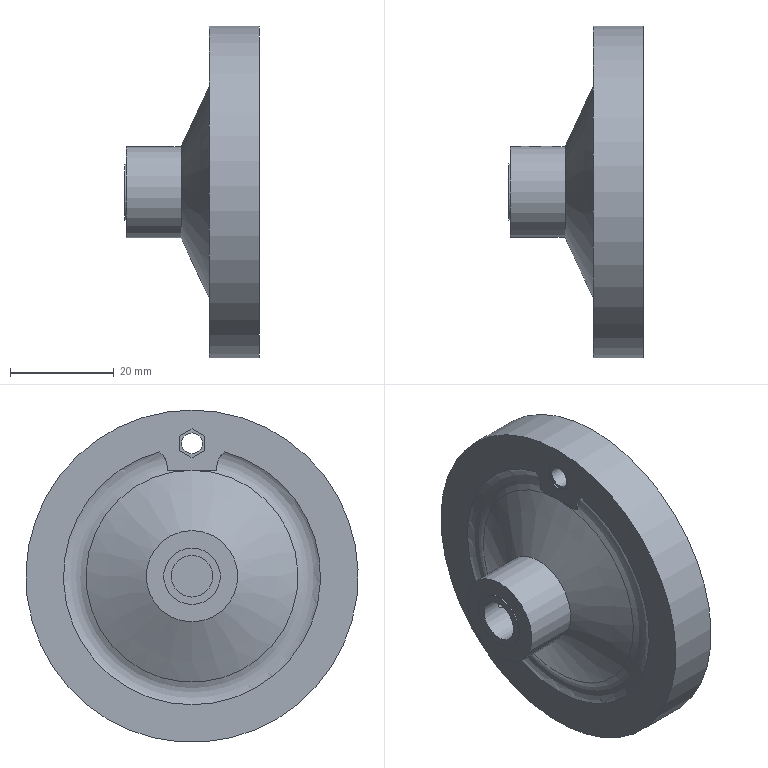Part | NX | features BREP 1 | 1 solid | 38 faces | box 25.84 x 64 x 64 mm | volume 22076 mm3 | plane 22 | cylinder 12 | torus 2 | cone 2 | commonest cylinder face diameters 8 x5 2.4 x1 4 x1 10.88 x1 12.8 x1 17.6 x1
STEP:
#1=CARTESIAN_POINT('',(-9.6,0.,22.829));
#2=VERTEX_POINT('',#1);
#3=CARTESIAN_POINT('',(-9.6,2.4,24.214));
#4=VERTEX_POINT('',#3);
#5=CARTESIAN_POINT('',(-9.6,3.971,25.122));
#6=DIRECTION('',(0.,0.866,0.5));
#7=VECTOR('',#6,1000.);
#8=LINE('',#5,#7);
#9=EDGE_CURVE('',#2,#4,#8,.T.);
#10=ORIENTED_EDGE('',*,*,#9,.F.);
#11=CARTESIAN_POINT('',(-9.36,0.,22.829));
#12=VERTEX_POINT('',#11);
#13=CARTESIAN_POINT('',(-9.36,0.,22.829));
#14=DIRECTION('',(-1.,0.,0.));
#15=VECTOR('',#14,1000.);
#16=LINE('',#13,#15);
#17=EDGE_CURVE('',#12,#2,#16,.T.);
#18=ORIENTED_EDGE('',*,*,#17,.F.);
#19=CARTESIAN_POINT('',(-9.36,2.4,24.214));
#20=VERTEX_POINT('',#19);
#21=CARTESIAN_POINT('',(-9.36,0.,22.829));
#22=DIRECTION('',(0.,0.866,0.5));
#23=VECTOR('',#22,1000.);
#24=LINE('',#21,#23);
#25=EDGE_CURVE('',#12,#20,#24,.T.);
#26=ORIENTED_EDGE('',*,*,#25,.T.);
#27=CARTESIAN_POINT('',(-9.36,2.4,24.214));
#28=DIRECTION('',(-1.,0.,0.));
#29=VECTOR('',#28,1000.);
#30=LINE('',#27,#29);
#31=EDGE_CURVE('',#20,#4,#30,.T.);
#32=ORIENTED_EDGE('',*,*,#31,.T.);
#33=EDGE_LOOP('',(#10,#18,#26,#32));
#34=FACE_BOUND('',#33,.T.);
#35=CARTESIAN_POINT('',(-9.36,0.,22.829));
#36=DIRECTION('',(0.,0.5,-0.866));
#37=DIRECTION('',(0.,-0.866,-0.5));
#38=AXIS2_PLACEMENT_3D('',#35,#36,#37);
#39=PLANE('',#38);
#40=ADVANCED_FACE('',(#34),#39,.F.);
#41=CARTESIAN_POINT('',(-9.6,2.4,26.986));
#42=VERTEX_POINT('',#41);
#43=CARTESIAN_POINT('',(-9.6,2.4,32.));
#44=DIRECTION('',(0.,0.,1.));
#45=VECTOR('',#44,1000.);
#46=LINE('',#43,#45);
#47=EDGE_CURVE('',#4,#42,#46,.T.);
#48=ORIENTED_EDGE('',*,*,#47,.F.);
#49=ORIENTED_EDGE('',*,*,#31,.F.);
#50=CARTESIAN_POINT('',(-9.36,2.4,26.986));
#51=VERTEX_POINT('',#50);
#52=CARTESIAN_POINT('',(-9.36,2.4,24.214));
#53=DIRECTION('',(0.,0.,1.));
#54=VECTOR('',#53,1000.);
#55=LINE('',#52,#54);
#56=EDGE_CURVE('',#20,#51,#55,.T.);
#57=ORIENTED_EDGE('',*,*,#56,.T.);
#58=CARTESIAN_POINT('',(-9.36,2.4,26.986));
#59=DIRECTION('',(-1.,0.,0.));
#60=VECTOR('',#59,1000.);
#61=LINE('',#58,#60);
#62=EDGE_CURVE('',#51,#42,#61,.T.);
#63=ORIENTED_EDGE('',*,*,#62,.T.);
#64=EDGE_LOOP('',(#48,#49,#57,#63));
#65=FACE_BOUND('',#64,.T.);
#66=CARTESIAN_POINT('',(-9.36,2.4,24.214));
#67=DIRECTION('',(0.,1.,0.));
#68=DIRECTION('',(0.,0.,-1.));
#69=AXIS2_PLACEMENT_3D('',#66,#67,#68);
#70=PLANE('',#69);
#71=ADVANCED_FACE('',(#65),#70,.F.);
#72=CARTESIAN_POINT('',(-9.6,0.,28.371));
#73=VERTEX_POINT('',#72);
#74=CARTESIAN_POINT('',(-9.6,-1.571,29.278));
#75=DIRECTION('',(0.,-0.866,0.5));
#76=VECTOR('',#75,1000.);
#77=LINE('',#74,#76);
#78=EDGE_CURVE('',#42,#73,#77,.T.);
#79=ORIENTED_EDGE('',*,*,#78,.F.);
#80=ORIENTED_EDGE('',*,*,#62,.F.);
#81=CARTESIAN_POINT('',(-9.36,0.,28.371));
#82=VERTEX_POINT('',#81);
#83=CARTESIAN_POINT('',(-9.36,2.4,26.986));
#84=DIRECTION('',(0.,-0.866,0.5));
#85=VECTOR('',#84,1000.);
#86=LINE('',#83,#85);
#87=EDGE_CURVE('',#51,#82,#86,.T.);
#88=ORIENTED_EDGE('',*,*,#87,.T.);
#89=CARTESIAN_POINT('',(-9.36,0.,28.371));
#90=DIRECTION('',(-1.,0.,0.));
#91=VECTOR('',#90,1000.);
#92=LINE('',#89,#91);
#93=EDGE_CURVE('',#82,#73,#92,.T.);
#94=ORIENTED_EDGE('',*,*,#93,.T.);
#95=EDGE_LOOP('',(#79,#80,#88,#94));
#96=FACE_BOUND('',#95,.T.);
#97=CARTESIAN_POINT('',(-9.36,2.4,26.986));
#98=DIRECTION('',(0.,0.5,0.866));
#99=DIRECTION('',(0.,0.866,-0.5));
#100=AXIS2_PLACEMENT_3D('',#97,#98,#99);
#101=PLANE('',#100);
#102=ADVANCED_FACE('',(#96),#101,.F.);
#103=CARTESIAN_POINT('',(-9.36,0.,27.6));
#104=VERTEX_POINT('',#103);
#105=CARTESIAN_POINT('',(-9.36,0.,25.6));
#106=DIRECTION('',(-1.,0.,0.));
#107=DIRECTION('',(0.,0.,1.));
#108=AXIS2_PLACEMENT_3D('',#105,#106,#107);
#109=CIRCLE('',#108,2.);
#110=EDGE_CURVE('',#104,#104,#109,.T.);
#111=ORIENTED_EDGE('',*,*,#110,.F.);
#112=EDGE_LOOP('',(#111));
#113=FACE_BOUND('',#112,.T.);
#114=CARTESIAN_POINT('',(-9.36,-2.4,26.986));
#115=VERTEX_POINT('',#114);
#116=CARTESIAN_POINT('',(-9.36,-2.4,24.214));
#117=VERTEX_POINT('',#116);
#118=CARTESIAN_POINT('',(-9.36,-2.4,26.986));
#119=DIRECTION('',(0.,0.,-1.));
#120=VECTOR('',#119,1000.);
#121=LINE('',#118,#120);
#122=EDGE_CURVE('',#115,#117,#121,.T.);
#123=ORIENTED_EDGE('',*,*,#122,.F.);
#124=CARTESIAN_POINT('',(-9.36,0.,28.371));
#125=DIRECTION('',(0.,-0.866,-0.5));
#126=VECTOR('',#125,1000.);
#127=LINE('',#124,#126);
#128=EDGE_CURVE('',#82,#115,#127,.T.);
#129=ORIENTED_EDGE('',*,*,#128,.F.);
#130=ORIENTED_EDGE('',*,*,#87,.F.);
#131=ORIENTED_EDGE('',*,*,#56,.F.);
#132=ORIENTED_EDGE('',*,*,#25,.F.);
#133=CARTESIAN_POINT('',(-9.36,-2.4,24.214));
#134=DIRECTION('',(0.,0.866,-0.5));
#135=VECTOR('',#134,1000.);
#136=LINE('',#133,#135);
#137=EDGE_CURVE('',#117,#12,#136,.T.);
#138=ORIENTED_EDGE('',*,*,#137,.F.);
#139=EDGE_LOOP('',(#123,#129,#130,#131,#132,#138));
#140=FACE_BOUND('',#139,.T.);
#141=CARTESIAN_POINT('',(-9.36,0.,0.));
#142=DIRECTION('',(-1.,0.,0.));
#143=DIRECTION('',(0.,0.,1.));
#144=AXIS2_PLACEMENT_3D('',#141,#142,#143);
#145=PLANE('',#144);
#146=ADVANCED_FACE('',(#113,#140),#145,.T.);
#147=CARTESIAN_POINT('',(-9.6,-2.4,26.986));
#148=VERTEX_POINT('',#147);
#149=CARTESIAN_POINT('',(-9.6,1.571,29.278));
#150=DIRECTION('',(0.,-0.866,-0.5));
#151=VECTOR('',#150,1000.);
#152=LINE('',#149,#151);
#153=EDGE_CURVE('',#73,#148,#152,.T.);
#154=ORIENTED_EDGE('',*,*,#153,.F.);
#155=ORIENTED_EDGE('',*,*,#93,.F.);
#156=ORIENTED_EDGE('',*,*,#128,.T.);
#157=CARTESIAN_POINT('',(-9.36,-2.4,26.986));
#158=DIRECTION('',(-1.,0.,0.));
#159=VECTOR('',#158,1000.);
#160=LINE('',#157,#159);
#161=EDGE_CURVE('',#115,#148,#160,.T.);
#162=ORIENTED_EDGE('',*,*,#161,.T.);
#163=EDGE_LOOP('',(#154,#155,#156,#162));
#164=FACE_BOUND('',#163,.T.);
#165=CARTESIAN_POINT('',(-9.36,0.,28.371));
#166=DIRECTION('',(0.,-0.5,0.866));
#167=DIRECTION('',(0.,0.866,0.5));
#168=AXIS2_PLACEMENT_3D('',#165,#166,#167);
#169=PLANE('',#168);
#170=ADVANCED_FACE('',(#164),#169,.F.);
#171=CARTESIAN_POINT('',(-9.6,-2.4,24.214));
#172=VERTEX_POINT('',#171);
#173=CARTESIAN_POINT('',(-9.6,-3.971,25.122));
#174=DIRECTION('',(0.,0.866,-0.5));
#175=VECTOR('',#174,1000.);
#176=LINE('',#173,#175);
#177=EDGE_CURVE('',#172,#2,#176,.T.);
#178=ORIENTED_EDGE('',*,*,#177,.F.);
#179=CARTESIAN_POINT('',(-9.36,-2.4,24.214));
#180=DIRECTION('',(-1.,0.,0.));
#181=VECTOR('',#180,1000.);
#182=LINE('',#179,#181);
#183=EDGE_CURVE('',#117,#172,#182,.T.);
#184=ORIENTED_EDGE('',*,*,#183,.F.);
#185=ORIENTED_EDGE('',*,*,#137,.T.);
#186=ORIENTED_EDGE('',*,*,#17,.T.);
#187=EDGE_LOOP('',(#178,#184,#185,#186));
#188=FACE_BOUND('',#187,.T.);
#189=CARTESIAN_POINT('',(-9.36,-2.4,24.214));
#190=DIRECTION('',(0.,-0.5,-0.866));
#191=DIRECTION('',(0.,-0.866,0.5));
#192=AXIS2_PLACEMENT_3D('',#189,#190,#191);
#193=PLANE('',#192);
#194=ADVANCED_FACE('',(#188),#193,.F.);
#195=ORIENTED_EDGE('',*,*,#183,.T.);
#196=CARTESIAN_POINT('',(-9.6,-2.4,32.));
#197=DIRECTION('',(0.,0.,-1.));
#198=VECTOR('',#197,1000.);
#199=LINE('',#196,#198);
#200=EDGE_CURVE('',#148,#172,#199,.T.);
#201=ORIENTED_EDGE('',*,*,#200,.F.);
#202=ORIENTED_EDGE('',*,*,#161,.F.);
#203=ORIENTED_EDGE('',*,*,#122,.T.);
#204=EDGE_LOOP('',(#195,#201,#202,#203));
#205=FACE_BOUND('',#204,.T.);
#206=CARTESIAN_POINT('',(-9.36,-2.4,26.986));
#207=DIRECTION('',(0.,-1.,0.));
#208=DIRECTION('',(0.,0.,1.));
#209=AXIS2_PLACEMENT_3D('',#206,#207,#208);
#210=PLANE('',#209);
#211=ADVANCED_FACE('',(#205),#210,.F.);
#212=CARTESIAN_POINT('',(-9.6,0.,10.208));
#213=VERTEX_POINT('',#212);
#214=CARTESIAN_POINT('',(-9.6,0.,0.));
#215=DIRECTION('',(-1.,0.,0.));
#216=DIRECTION('',(0.,0.,1.));
#217=AXIS2_PLACEMENT_3D('',#214,#215,#216);
#218=CIRCLE('',#217,10.208);
#219=EDGE_CURVE('',#213,#213,#218,.T.);
#220=ORIENTED_EDGE('',*,*,#219,.F.);
#221=EDGE_LOOP('',(#220));
#222=FACE_BOUND('',#221,.T.);
#223=CARTESIAN_POINT('',(-9.6,0.,0.));
#224=DIRECTION('',(-1.,0.,0.));
#225=DIRECTION('',(0.,0.,-1.));
#226=AXIS2_PLACEMENT_3D('',#223,#224,#225);
#227=PLANE('',#226);
#228=ADVANCED_FACE('',(#222),#227,.F.);
#229=CARTESIAN_POINT('',(-12.8,0.,4.));
#230=VERTEX_POINT('',#229);
#231=CARTESIAN_POINT('',(-12.8,0.,0.));
#232=DIRECTION('',(-1.,0.,0.));
#233=DIRECTION('',(0.,0.,1.));
#234=AXIS2_PLACEMENT_3D('',#231,#232,#233);
#235=CIRCLE('',#234,4.);
#236=EDGE_CURVE('',#230,#230,#235,.T.);
#237=ORIENTED_EDGE('',*,*,#236,.T.);
#238=EDGE_LOOP('',(#237));
#239=FACE_BOUND('',#238,.T.);
#240=CARTESIAN_POINT('',(-12.8,0.,4.));
#241=DIRECTION('',(1.,0.,0.));
#242=DIRECTION('',(0.,0.,1.));
#243=AXIS2_PLACEMENT_3D('',#240,#241,#242);
#244=PLANE('',#243);
#245=ADVANCED_FACE('',(#239),#244,.F.);
#246=CARTESIAN_POINT('',(-25.84,0.,4.));
#247=VERTEX_POINT('',#246);
#248=CARTESIAN_POINT('',(-25.84,0.,0.));
#249=DIRECTION('',(-1.,0.,0.));
#250=DIRECTION('',(0.,0.,1.));
#251=AXIS2_PLACEMENT_3D('',#248,#249,#250);
#252=CIRCLE('',#251,4.);
#253=EDGE_CURVE('',#247,#247,#252,.T.);
#254=ORIENTED_EDGE('',*,*,#253,.F.);
#255=EDGE_LOOP('',(#254));
#256=FACE_BOUND('',#255,.T.);
#257=CARTESIAN_POINT('',(-25.84,0.,5.44));
#258=VERTEX_POINT('',#257);
#259=CARTESIAN_POINT('',(-25.84,0.,0.));
#260=DIRECTION('',(-1.,0.,0.));
#261=DIRECTION('',(0.,0.,1.));
#262=AXIS2_PLACEMENT_3D('',#259,#260,#261);
#263=CIRCLE('',#262,5.44);
#264=EDGE_CURVE('',#258,#258,#263,.T.);
#265=ORIENTED_EDGE('',*,*,#264,.T.);
#266=EDGE_LOOP('',(#265));
#267=FACE_BOUND('',#266,.T.);
#268=CARTESIAN_POINT('',(-25.84,0.,5.44));
#269=DIRECTION('',(1.,0.,0.));
#270=DIRECTION('',(0.,0.,1.));
#271=AXIS2_PLACEMENT_3D('',#268,#269,#270);
#272=PLANE('',#271);
#273=ADVANCED_FACE('',(#256,#267),#272,.F.);
#274=CARTESIAN_POINT('',(-9.6,0.,12.848));
#275=VERTEX_POINT('',#274);
#276=CARTESIAN_POINT('',(-9.6,0.,0.));
#277=DIRECTION('',(-1.,0.,0.));
#278=DIRECTION('',(0.,0.,1.));
#279=AXIS2_PLACEMENT_3D('',#276,#277,#278);
#280=CIRCLE('',#279,12.848);
#281=EDGE_CURVE('',#275,#275,#280,.T.);
#282=ORIENTED_EDGE('',*,*,#281,.F.);
#283=EDGE_LOOP('',(#282));
#284=FACE_BOUND('',#283,.T.);
#285=ORIENTED_EDGE('',*,*,#219,.T.);
#286=EDGE_LOOP('',(#285));
#287=FACE_BOUND('',#286,.T.);
#288=CARTESIAN_POINT('',(-6.769,0.,0.));
#289=DIRECTION('',(-1.,0.,0.));
#290=DIRECTION('',(0.,0.,-1.));
#291=AXIS2_PLACEMENT_3D('',#288,#289,#290);
#292=TOROIDAL_SURFACE('',#291,11.528,3.123);
#293=ADVANCED_FACE('',(#284,#287),#292,.F.);
#294=ORIENTED_EDGE('',*,*,#236,.F.);
#295=EDGE_LOOP('',(#294));
#296=FACE_BOUND('',#295,.T.);
#297=ORIENTED_EDGE('',*,*,#253,.T.);
#298=EDGE_LOOP('',(#297));
#299=FACE_BOUND('',#298,.T.);
#300=CARTESIAN_POINT('',(-20.8,3.816,-1.2));
#301=VERTEX_POINT('',#300);
#302=CARTESIAN_POINT('',(-21.741,3.91,-0.9399));
#303=CARTESIAN_POINT('',(-20.8,3.769,-1.33));
#304=CARTESIAN_POINT('',(-19.86,3.91,-0.9398));
#305=CARTESIAN_POINT('',(-19.47,4.045,-0.001488));
#306=CARTESIAN_POINT('',(-19.86,3.91,0.941));
#307=CARTESIAN_POINT('',(-20.799,3.769,1.329));
#308=CARTESIAN_POINT('',(-21.74,3.91,0.9411));
#309=CARTESIAN_POINT('',(-22.13,4.045,0.0001827));
#310=CARTESIAN_POINT('',(-21.741,3.91,-0.9399));
#311=CARTESIAN_POINT('',(-20.8,3.769,-1.33));
#312=CARTESIAN_POINT('',(-19.86,3.91,-0.9398));
#313=B_SPLINE_CURVE_WITH_KNOTS('',3,(#302,#303,#304,#305,#306,#307,#308,#309,#310,#311,#312),.UNSPECIFIED.,.T.,.F.,(1,1,1,1,1,1,1,1,1,1,1,1,1,1,1),(-0.00283,-0.001887,-0.0009433,0.,0.0009433,0.001887,0.00283,0.003773,0.004716,0.00566,0.006603,0.007546,0.008489,0.009433,0.01038),.UNSPECIFIED.);
#314=EDGE_CURVE('',#301,#301,#313,.T.);
#315=ORIENTED_EDGE('',*,*,#314,.F.);
#316=EDGE_LOOP('',(#315));
#317=FACE_BOUND('',#316,.T.);
#318=CARTESIAN_POINT('',(0.,0.,0.));
#319=DIRECTION('',(-1.,0.,0.));
#320=DIRECTION('',(0.,0.,-1.));
#321=AXIS2_PLACEMENT_3D('',#318,#319,#320);
#322=CYLINDRICAL_SURFACE('',#321,4.);
#323=ADVANCED_FACE('',(#296,#299,#317),#322,.F.);
#324=ORIENTED_EDGE('',*,*,#264,.F.);
#325=EDGE_LOOP('',(#324));
#326=FACE_BOUND('',#325,.T.);
#327=CARTESIAN_POINT('',(-25.6,0.,5.44));
#328=VERTEX_POINT('',#327);
#329=CARTESIAN_POINT('',(-25.6,0.,0.));
#330=DIRECTION('',(-1.,0.,0.));
#331=DIRECTION('',(0.,0.,1.));
#332=AXIS2_PLACEMENT_3D('',#329,#330,#331);
#333=CIRCLE('',#332,5.44);
#334=EDGE_CURVE('',#328,#328,#333,.T.);
#335=ORIENTED_EDGE('',*,*,#334,.T.);
#336=EDGE_LOOP('',(#335));
#337=FACE_BOUND('',#336,.T.);
#338=CARTESIAN_POINT('',(0.,0.,0.));
#339=DIRECTION('',(-1.,0.,0.));
#340=DIRECTION('',(0.,0.,-1.));
#341=AXIS2_PLACEMENT_3D('',#338,#339,#340);
#342=CYLINDRICAL_SURFACE('',#341,5.44);
#343=ADVANCED_FACE('',(#326,#337),#342,.T.);
#344=CARTESIAN_POINT('',(-5.132,5.168,21.825));
#345=VERTEX_POINT('',#344);
#346=CARTESIAN_POINT('',(-3.84,9.983,23.138));
#347=VERTEX_POINT('',#346);
#348=CARTESIAN_POINT('',(-5.132,5.168,21.825));
#349=CARTESIAN_POINT('',(-4.762,5.677,22.521));
#350=CARTESIAN_POINT('',(-4.11,7.161,23.596));
#351=CARTESIAN_POINT('',(-3.84,9.119,23.511));
#352=CARTESIAN_POINT('',(-3.84,9.983,23.138));
#353=B_SPLINE_CURVE_WITH_KNOTS('',3,(#348,#349,#350,#351,#352),.UNSPECIFIED.,.F.,.F.,(4,1,4),(0.,0.002777,0.005554),.UNSPECIFIED.);
#354=EDGE_CURVE('',#345,#347,#353,.T.);
#355=ORIENTED_EDGE('',*,*,#354,.F.);
#356=CARTESIAN_POINT('',(-5.132,-5.168,21.825));
#357=VERTEX_POINT('',#356);
#358=CARTESIAN_POINT('',(-5.132,-5.168,21.825));
#359=CARTESIAN_POINT('',(-5.546,-4.6,21.047));
#360=CARTESIAN_POINT('',(-6.299,-3.109,19.734));
#361=CARTESIAN_POINT('',(-6.806,-0.0188,18.935));
#362=CARTESIAN_POINT('',(-6.303,3.107,19.728));
#363=CARTESIAN_POINT('',(-5.547,4.599,21.046));
#364=CARTESIAN_POINT('',(-5.132,5.168,21.825));
#365=B_SPLINE_CURVE_WITH_KNOTS('',3,(#358,#359,#360,#361,#362,#363,#364),.UNSPECIFIED.,.F.,.F.,(4,1,1,1,4),(0.,0.003106,0.006212,0.009318,0.01242),.UNSPECIFIED.);
#366=EDGE_CURVE('',#357,#345,#365,.T.);
#367=ORIENTED_EDGE('',*,*,#366,.F.);
#368=CARTESIAN_POINT('',(-3.84,-9.983,23.138));
#369=VERTEX_POINT('',#368);
#370=CARTESIAN_POINT('',(-3.84,-9.983,23.138));
#371=CARTESIAN_POINT('',(-3.84,-9.121,23.51));
#372=CARTESIAN_POINT('',(-4.108,-7.168,23.599));
#373=CARTESIAN_POINT('',(-4.762,-5.676,22.52));
#374=CARTESIAN_POINT('',(-5.132,-5.168,21.825));
#375=B_SPLINE_CURVE_WITH_KNOTS('',3,(#370,#371,#372,#373,#374),.UNSPECIFIED.,.F.,.F.,(4,1,4),(0.,0.002776,0.005551),.UNSPECIFIED.);
#376=EDGE_CURVE('',#369,#357,#375,.T.);
#377=ORIENTED_EDGE('',*,*,#376,.F.);
#378=CARTESIAN_POINT('',(-3.84,0.,0.));
#379=DIRECTION('',(-1.,0.,0.));
#380=DIRECTION('',(0.,0.,1.));
#381=AXIS2_PLACEMENT_3D('',#378,#379,#380);
#382=CIRCLE('',#381,25.2);
#383=EDGE_CURVE('',#347,#369,#382,.T.);
#384=ORIENTED_EDGE('',*,*,#383,.F.);
#385=EDGE_LOOP('',(#355,#367,#377,#384));
#386=FACE_BOUND('',#385,.T.);
#387=ORIENTED_EDGE('',*,*,#281,.T.);
#388=EDGE_LOOP('',(#387));
#389=FACE_BOUND('',#388,.T.);
#390=CARTESIAN_POINT('',(-9.6,0.,0.));
#391=DIRECTION('',(1.,0.,0.));
#392=DIRECTION('',(0.,0.,1.));
#393=AXIS2_PLACEMENT_3D('',#390,#391,#392);
#394=CONICAL_SURFACE('',#393,12.848,1.134);
#395=ADVANCED_FACE('',(#386,#389),#394,.F.);
#396=CARTESIAN_POINT('',(-20.8,8.718,-1.2));
#397=VERTEX_POINT('',#396);
#398=CARTESIAN_POINT('',(-19.859,8.759,-0.9396));
#399=CARTESIAN_POINT('',(-20.8,8.697,-1.33));
#400=CARTESIAN_POINT('',(-21.74,8.759,-0.9398));
#401=CARTESIAN_POINT('',(-22.13,8.82,-0.001097));
#402=CARTESIAN_POINT('',(-21.741,8.759,0.9402));
#403=CARTESIAN_POINT('',(-20.8,8.697,1.33));
#404=CARTESIAN_POINT('',(-19.861,8.759,0.9413));
#405=CARTESIAN_POINT('',(-19.47,8.82,0.001145));
#406=CARTESIAN_POINT('',(-19.859,8.759,-0.9396));
#407=CARTESIAN_POINT('',(-20.8,8.697,-1.33));
#408=CARTESIAN_POINT('',(-21.74,8.759,-0.9398));
#409=B_SPLINE_CURVE_WITH_KNOTS('',3,(#398,#399,#400,#401,#402,#403,#404,#405,#406,#407,#408),.UNSPECIFIED.,.T.,.F.,(1,1,1,1,1,1,1,1,1,1,1,1,1,1,1),(-0.002817,-0.001878,-0.0009389,0.,0.0009389,0.001878,0.002817,0.003756,0.004695,0.005633,0.006572,0.007511,0.00845,0.009389,0.01033),.UNSPECIFIED.);
#410=EDGE_CURVE('',#397,#397,#409,.T.);
#411=ORIENTED_EDGE('',*,*,#410,.T.);
#412=EDGE_LOOP('',(#411));
#413=FACE_BOUND('',#412,.T.);
#414=ORIENTED_EDGE('',*,*,#314,.T.);
#415=EDGE_LOOP('',(#414));
#416=FACE_BOUND('',#415,.T.);
#417=CARTESIAN_POINT('',(-20.8,94.126,0.));
#418=DIRECTION('',(0.,-1.,0.));
#419=DIRECTION('',(0.,0.,1.));
#420=AXIS2_PLACEMENT_3D('',#417,#418,#419);
#421=CYLINDRICAL_SURFACE('',#420,1.2);
#422=ADVANCED_FACE('',(#413,#416),#421,.F.);
#423=ORIENTED_EDGE('',*,*,#334,.F.);
#424=EDGE_LOOP('',(#423));
#425=FACE_BOUND('',#424,.T.);
#426=CARTESIAN_POINT('',(-25.6,0.,8.8));
#427=VERTEX_POINT('',#426);
#428=CARTESIAN_POINT('',(-25.6,0.,0.));
#429=DIRECTION('',(-1.,0.,0.));
#430=DIRECTION('',(0.,0.,1.));
#431=AXIS2_PLACEMENT_3D('',#428,#429,#430);
#432=CIRCLE('',#431,8.8);
#433=EDGE_CURVE('',#427,#427,#432,.T.);
#434=ORIENTED_EDGE('',*,*,#433,.T.);
#435=EDGE_LOOP('',(#434));
#436=FACE_BOUND('',#435,.T.);
#437=CARTESIAN_POINT('',(-25.6,0.,5.44));
#438=DIRECTION('',(1.,0.,0.));
#439=DIRECTION('',(0.,0.,1.));
#440=AXIS2_PLACEMENT_3D('',#437,#438,#439);
#441=PLANE('',#440);
#442=ADVANCED_FACE('',(#425,#436),#441,.F.);
#443=CARTESIAN_POINT('',(0.,0.,28.371));
#444=VERTEX_POINT('',#443);
#445=CARTESIAN_POINT('',(0.,-2.4,26.986));
#446=VERTEX_POINT('',#445);
#447=CARTESIAN_POINT('',(0.,0.,28.371));
#448=DIRECTION('',(0.,-0.866,-0.5));
#449=VECTOR('',#448,1000.);
#450=LINE('',#447,#449);
#451=EDGE_CURVE('',#444,#446,#450,.T.);
#452=ORIENTED_EDGE('',*,*,#451,.T.);
#453=CARTESIAN_POINT('',(-0.24,-2.4,26.986));
#454=VERTEX_POINT('',#453);
#455=CARTESIAN_POINT('',(-0.24,-2.4,26.986));
#456=DIRECTION('',(1.,0.,0.));
#457=VECTOR('',#456,1000.);
#458=LINE('',#455,#457);
#459=EDGE_CURVE('',#454,#446,#458,.T.);
#460=ORIENTED_EDGE('',*,*,#459,.F.);
#461=CARTESIAN_POINT('',(-0.24,0.,28.371));
#462=VERTEX_POINT('',#461);
#463=CARTESIAN_POINT('',(-0.24,0.,28.371));
#464=DIRECTION('',(0.,-0.866,-0.5));
#465=VECTOR('',#464,1000.);
#466=LINE('',#463,#465);
#467=EDGE_CURVE('',#462,#454,#466,.T.);
#468=ORIENTED_EDGE('',*,*,#467,.F.);
#469=CARTESIAN_POINT('',(-0.24,0.,28.371));
#470=DIRECTION('',(1.,0.,0.));
#471=VECTOR('',#470,1000.);
#472=LINE('',#469,#471);
#473=EDGE_CURVE('',#462,#444,#472,.T.);
#474=ORIENTED_EDGE('',*,*,#473,.T.);
#475=EDGE_LOOP('',(#452,#460,#468,#474));
#476=FACE_BOUND('',#475,.T.);
#477=CARTESIAN_POINT('',(-0.24,0.,28.371));
#478=DIRECTION('',(0.,-0.5,0.866));
#479=DIRECTION('',(0.,0.866,0.5));
#480=AXIS2_PLACEMENT_3D('',#477,#478,#479);
#481=PLANE('',#480);
#482=ADVANCED_FACE('',(#476),#481,.F.);
#483=CARTESIAN_POINT('',(0.,2.4,26.986));
#484=VERTEX_POINT('',#483);
#485=CARTESIAN_POINT('',(0.,2.4,26.986));
#486=DIRECTION('',(0.,-0.866,0.5));
#487=VECTOR('',#486,1000.);
#488=LINE('',#485,#487);
#489=EDGE_CURVE('',#484,#444,#488,.T.);
#490=ORIENTED_EDGE('',*,*,#489,.T.);
#491=ORIENTED_EDGE('',*,*,#473,.F.);
#492=CARTESIAN_POINT('',(-0.24,2.4,26.986));
#493=VERTEX_POINT('',#492);
#494=CARTESIAN_POINT('',(-0.24,2.4,26.986));
#495=DIRECTION('',(0.,-0.866,0.5));
#496=VECTOR('',#495,1000.);
#497=LINE('',#494,#496);
#498=EDGE_CURVE('',#493,#462,#497,.T.);
#499=ORIENTED_EDGE('',*,*,#498,.F.);
#500=CARTESIAN_POINT('',(-0.24,2.4,26.986));
#501=DIRECTION('',(1.,0.,0.));
#502=VECTOR('',#501,1000.);
#503=LINE('',#500,#502);
#504=EDGE_CURVE('',#493,#484,#503,.T.);
#505=ORIENTED_EDGE('',*,*,#504,.T.);
#506=EDGE_LOOP('',(#490,#491,#499,#505));
#507=FACE_BOUND('',#506,.T.);
#508=CARTESIAN_POINT('',(-0.24,2.4,26.986));
#509=DIRECTION('',(0.,0.5,0.866));
#510=DIRECTION('',(0.,0.866,-0.5));
#511=AXIS2_PLACEMENT_3D('',#508,#509,#510);
#512=PLANE('',#511);
#513=ADVANCED_FACE('',(#507),#512,.F.);
#514=CARTESIAN_POINT('',(0.,2.4,24.214));
#515=VERTEX_POINT('',#514);
#516=CARTESIAN_POINT('',(0.,2.4,24.214));
#517=DIRECTION('',(0.,0.,1.));
#518=VECTOR('',#517,1000.);
#519=LINE('',#516,#518);
#520=EDGE_CURVE('',#515,#484,#519,.T.);
#521=ORIENTED_EDGE('',*,*,#520,.T.);
#522=ORIENTED_EDGE('',*,*,#504,.F.);
#523=CARTESIAN_POINT('',(-0.24,2.4,24.214));
#524=VERTEX_POINT('',#523);
#525=CARTESIAN_POINT('',(-0.24,2.4,24.214));
#526=DIRECTION('',(0.,0.,1.));
#527=VECTOR('',#526,1000.);
#528=LINE('',#525,#527);
#529=EDGE_CURVE('',#524,#493,#528,.T.);
#530=ORIENTED_EDGE('',*,*,#529,.F.);
#531=CARTESIAN_POINT('',(-0.24,2.4,24.214));
#532=DIRECTION('',(1.,0.,0.));
#533=VECTOR('',#532,1000.);
#534=LINE('',#531,#533);
#535=EDGE_CURVE('',#524,#515,#534,.T.);
#536=ORIENTED_EDGE('',*,*,#535,.T.);
#537=EDGE_LOOP('',(#521,#522,#530,#536));
#538=FACE_BOUND('',#537,.T.);
#539=CARTESIAN_POINT('',(-0.24,2.4,24.214));
#540=DIRECTION('',(0.,1.,0.));
#541=DIRECTION('',(0.,0.,-1.));
#542=AXIS2_PLACEMENT_3D('',#539,#540,#541);
#543=PLANE('',#542);
#544=ADVANCED_FACE('',(#538),#543,.F.);
#545=CARTESIAN_POINT('',(0.,0.,22.829));
#546=VERTEX_POINT('',#545);
#547=CARTESIAN_POINT('',(0.,0.,22.829));
#548=DIRECTION('',(0.,0.866,0.5));
#549=VECTOR('',#548,1000.);
#550=LINE('',#547,#549);
#551=EDGE_CURVE('',#546,#515,#550,.T.);
#552=ORIENTED_EDGE('',*,*,#551,.T.);
#553=ORIENTED_EDGE('',*,*,#535,.F.);
#554=CARTESIAN_POINT('',(-0.24,0.,22.829));
#555=VERTEX_POINT('',#554);
#556=CARTESIAN_POINT('',(-0.24,0.,22.829));
#557=DIRECTION('',(0.,0.866,0.5));
#558=VECTOR('',#557,1000.);
#559=LINE('',#556,#558);
#560=EDGE_CURVE('',#555,#524,#559,.T.);
#561=ORIENTED_EDGE('',*,*,#560,.F.);
#562=CARTESIAN_POINT('',(-0.24,0.,22.829));
#563=DIRECTION('',(1.,0.,0.));
#564=VECTOR('',#563,1000.);
#565=LINE('',#562,#564);
#566=EDGE_CURVE('',#555,#546,#565,.T.);
#567=ORIENTED_EDGE('',*,*,#566,.T.);
#568=EDGE_LOOP('',(#552,#553,#561,#567));
#569=FACE_BOUND('',#568,.T.);
#570=CARTESIAN_POINT('',(-0.24,0.,22.829));
#571=DIRECTION('',(0.,0.5,-0.866));
#572=DIRECTION('',(0.,-0.866,-0.5));
#573=AXIS2_PLACEMENT_3D('',#570,#571,#572);
#574=PLANE('',#573);
#575=ADVANCED_FACE('',(#569),#574,.F.);
#576=CARTESIAN_POINT('',(0.,-2.4,24.214));
#577=VERTEX_POINT('',#576);
#578=CARTESIAN_POINT('',(0.,-2.4,24.214));
#579=DIRECTION('',(0.,0.866,-0.5));
#580=VECTOR('',#579,1000.);
#581=LINE('',#578,#580);
#582=EDGE_CURVE('',#577,#546,#581,.T.);
#583=ORIENTED_EDGE('',*,*,#582,.T.);
#584=ORIENTED_EDGE('',*,*,#566,.F.);
#585=CARTESIAN_POINT('',(-0.24,-2.4,24.214));
#586=VERTEX_POINT('',#585);
#587=CARTESIAN_POINT('',(-0.24,-2.4,24.214));
#588=DIRECTION('',(0.,0.866,-0.5));
#589=VECTOR('',#588,1000.);
#590=LINE('',#587,#589);
#591=EDGE_CURVE('',#586,#555,#590,.T.);
#592=ORIENTED_EDGE('',*,*,#591,.F.);
#593=CARTESIAN_POINT('',(-0.24,-2.4,24.214));
#594=DIRECTION('',(1.,0.,0.));
#595=VECTOR('',#594,1000.);
#596=LINE('',#593,#595);
#597=EDGE_CURVE('',#586,#577,#596,.T.);
#598=ORIENTED_EDGE('',*,*,#597,.T.);
#599=EDGE_LOOP('',(#583,#584,#592,#598));
#600=FACE_BOUND('',#599,.T.);
#601=CARTESIAN_POINT('',(-0.24,-2.4,24.214));
#602=DIRECTION('',(0.,-0.5,-0.866));
#603=DIRECTION('',(0.,-0.866,0.5));
#604=AXIS2_PLACEMENT_3D('',#601,#602,#603);
#605=PLANE('',#604);
#606=ADVANCED_FACE('',(#600),#605,.F.);
#607=ORIENTED_EDGE('',*,*,#597,.F.);
#608=CARTESIAN_POINT('',(-0.24,-2.4,26.986));
#609=DIRECTION('',(0.,0.,-1.));
#610=VECTOR('',#609,1000.);
#611=LINE('',#608,#610);
#612=EDGE_CURVE('',#454,#586,#611,.T.);
#613=ORIENTED_EDGE('',*,*,#612,.F.);
#614=ORIENTED_EDGE('',*,*,#459,.T.);
#615=CARTESIAN_POINT('',(0.,-2.4,26.986));
#616=DIRECTION('',(0.,0.,-1.));
#617=VECTOR('',#616,1000.);
#618=LINE('',#615,#617);
#619=EDGE_CURVE('',#446,#577,#618,.T.);
#620=ORIENTED_EDGE('',*,*,#619,.T.);
#621=EDGE_LOOP('',(#607,#613,#614,#620));
#622=FACE_BOUND('',#621,.T.);
#623=CARTESIAN_POINT('',(-0.24,-2.4,26.986));
#624=DIRECTION('',(0.,-1.,0.));
#625=DIRECTION('',(0.,0.,1.));
#626=AXIS2_PLACEMENT_3D('',#623,#624,#625);
#627=PLANE('',#626);
#628=ADVANCED_FACE('',(#622),#627,.F.);
#629=CARTESIAN_POINT('',(-0.24,0.,23.6));
#630=VERTEX_POINT('',#629);
#631=CARTESIAN_POINT('',(-0.24,0.,25.6));
#632=DIRECTION('',(1.,0.,0.));
#633=DIRECTION('',(0.,0.,-1.));
#634=AXIS2_PLACEMENT_3D('',#631,#632,#633);
#635=CIRCLE('',#634,2.);
#636=EDGE_CURVE('',#630,#630,#635,.T.);
#637=ORIENTED_EDGE('',*,*,#636,.F.);
#638=EDGE_LOOP('',(#637));
#639=FACE_BOUND('',#638,.T.);
#640=ORIENTED_EDGE('',*,*,#612,.T.);
#641=ORIENTED_EDGE('',*,*,#591,.T.);
#642=ORIENTED_EDGE('',*,*,#560,.T.);
#643=ORIENTED_EDGE('',*,*,#529,.T.);
#644=ORIENTED_EDGE('',*,*,#498,.T.);
#645=ORIENTED_EDGE('',*,*,#467,.T.);
#646=EDGE_LOOP('',(#640,#641,#642,#643,#644,#645));
#647=FACE_BOUND('',#646,.T.);
#648=CARTESIAN_POINT('',(-0.24,0.,0.));
#649=DIRECTION('',(1.,0.,0.));
#650=DIRECTION('',(0.,0.,1.));
#651=AXIS2_PLACEMENT_3D('',#648,#649,#650);
#652=PLANE('',#651);
#653=ADVANCED_FACE('',(#639,#647),#652,.T.);
#654=ORIENTED_EDGE('',*,*,#636,.T.);
#655=EDGE_LOOP('',(#654));
#656=FACE_BOUND('',#655,.T.);
#657=ORIENTED_EDGE('',*,*,#110,.T.);
#658=EDGE_LOOP('',(#657));
#659=FACE_BOUND('',#658,.T.);
#660=CARTESIAN_POINT('',(-94.126,0.,25.6));
#661=DIRECTION('',(1.,0.,0.));
#662=DIRECTION('',(0.,0.,1.));
#663=AXIS2_PLACEMENT_3D('',#660,#661,#662);
#664=CYLINDRICAL_SURFACE('',#663,2.);
#665=ADVANCED_FACE('',(#656,#659),#664,.F.);
#666=CARTESIAN_POINT('',(0.,-9.983,23.138));
#667=VERTEX_POINT('',#666);
#668=CARTESIAN_POINT('',(-94.126,-9.983,23.138));
#669=DIRECTION('',(1.,0.,0.));
#670=VECTOR('',#669,1000.);
#671=LINE('',#668,#670);
#672=EDGE_CURVE('',#369,#667,#671,.T.);
#673=ORIENTED_EDGE('',*,*,#672,.T.);
#674=CARTESIAN_POINT('',(0.,9.983,23.138));
#675=VERTEX_POINT('',#674);
#676=CARTESIAN_POINT('',(0.,0.,0.));
#677=DIRECTION('',(-1.,0.,0.));
#678=DIRECTION('',(0.,0.,1.));
#679=AXIS2_PLACEMENT_3D('',#676,#677,#678);
#680=CIRCLE('',#679,25.2);
#681=EDGE_CURVE('',#675,#667,#680,.T.);
#682=ORIENTED_EDGE('',*,*,#681,.F.);
#683=CARTESIAN_POINT('',(-94.126,9.983,23.138));
#684=DIRECTION('',(1.,0.,0.));
#685=VECTOR('',#684,1000.);
#686=LINE('',#683,#685);
#687=EDGE_CURVE('',#347,#675,#686,.T.);
#688=ORIENTED_EDGE('',*,*,#687,.F.);
#689=ORIENTED_EDGE('',*,*,#383,.T.);
#690=EDGE_LOOP('',(#673,#682,#688,#689));
#691=FACE_BOUND('',#690,.T.);
#692=CARTESIAN_POINT('',(0.,0.,0.));
#693=DIRECTION('',(-1.,0.,0.));
#694=DIRECTION('',(0.,0.,-1.));
#695=AXIS2_PLACEMENT_3D('',#692,#693,#694);
#696=CYLINDRICAL_SURFACE('',#695,25.2);
#697=ADVANCED_FACE('',(#691),#696,.F.);
#698=CARTESIAN_POINT('',(0.,5.168,21.825));
#699=VERTEX_POINT('',#698);
#700=CARTESIAN_POINT('',(-94.126,5.168,21.825));
#701=DIRECTION('',(1.,0.,0.));
#702=VECTOR('',#701,1000.);
#703=LINE('',#700,#702);
#704=EDGE_CURVE('',#345,#699,#703,.T.);
#705=ORIENTED_EDGE('',*,*,#704,.F.);
#706=ORIENTED_EDGE('',*,*,#354,.T.);
#707=ORIENTED_EDGE('',*,*,#687,.T.);
#708=CARTESIAN_POINT('',(0.,8.398,19.466));
#709=DIRECTION('',(1.,0.,0.));
#710=DIRECTION('',(0.,1.,0.));
#711=AXIS2_PLACEMENT_3D('',#708,#709,#710);
#712=CIRCLE('',#711,4.);
#713=EDGE_CURVE('',#675,#699,#712,.T.);
#714=ORIENTED_EDGE('',*,*,#713,.T.);
#715=EDGE_LOOP('',(#705,#706,#707,#714));
#716=FACE_BOUND('',#715,.T.);
#717=CARTESIAN_POINT('',(-94.126,8.398,19.466));
#718=DIRECTION('',(1.,0.,0.));
#719=DIRECTION('',(0.,0.,1.));
#720=AXIS2_PLACEMENT_3D('',#717,#718,#719);
#721=CYLINDRICAL_SURFACE('',#720,4.);
#722=ADVANCED_FACE('',(#716),#721,.F.);
#723=ORIENTED_EDGE('',*,*,#366,.T.);
#724=ORIENTED_EDGE('',*,*,#704,.T.);
#725=CARTESIAN_POINT('',(0.,-5.168,21.825));
#726=VERTEX_POINT('',#725);
#727=CARTESIAN_POINT('',(0.,0.,25.6));
#728=DIRECTION('',(-1.,0.,0.));
#729=DIRECTION('',(0.,1.,0.));
#730=AXIS2_PLACEMENT_3D('',#727,#728,#729);
#731=CIRCLE('',#730,6.4);
#732=EDGE_CURVE('',#699,#726,#731,.T.);
#733=ORIENTED_EDGE('',*,*,#732,.T.);
#734=CARTESIAN_POINT('',(-94.126,-5.168,21.825));
#735=DIRECTION('',(1.,0.,0.));
#736=VECTOR('',#735,1000.);
#737=LINE('',#734,#736);
#738=EDGE_CURVE('',#357,#726,#737,.T.);
#739=ORIENTED_EDGE('',*,*,#738,.F.);
#740=EDGE_LOOP('',(#723,#724,#733,#739));
#741=FACE_BOUND('',#740,.T.);
#742=CARTESIAN_POINT('',(-94.126,0.,25.6));
#743=DIRECTION('',(1.,0.,0.));
#744=DIRECTION('',(0.,0.,1.));
#745=AXIS2_PLACEMENT_3D('',#742,#743,#744);
#746=CYLINDRICAL_SURFACE('',#745,6.4);
#747=ADVANCED_FACE('',(#741),#746,.T.);
#748=ORIENTED_EDGE('',*,*,#672,.F.);
#749=ORIENTED_EDGE('',*,*,#376,.T.);
#750=ORIENTED_EDGE('',*,*,#738,.T.);
#751=CARTESIAN_POINT('',(0.,-8.398,19.466));
#752=DIRECTION('',(1.,0.,0.));
#753=DIRECTION('',(0.,1.,0.));
#754=AXIS2_PLACEMENT_3D('',#751,#752,#753);
#755=CIRCLE('',#754,4.);
#756=EDGE_CURVE('',#726,#667,#755,.T.);
#757=ORIENTED_EDGE('',*,*,#756,.T.);
#758=EDGE_LOOP('',(#748,#749,#750,#757));
#759=FACE_BOUND('',#758,.T.);
#760=CARTESIAN_POINT('',(-94.126,-8.398,19.466));
#761=DIRECTION('',(1.,0.,0.));
#762=DIRECTION('',(0.,0.,1.));
#763=AXIS2_PLACEMENT_3D('',#760,#761,#762);
#764=CYLINDRICAL_SURFACE('',#763,4.);
#765=ADVANCED_FACE('',(#759),#764,.F.);
#766=ORIENTED_EDGE('',*,*,#433,.F.);
#767=EDGE_LOOP('',(#766));
#768=FACE_BOUND('',#767,.T.);
#769=CARTESIAN_POINT('',(-15.018,0.,8.8));
#770=VERTEX_POINT('',#769);
#771=CARTESIAN_POINT('',(-15.018,0.,0.));
#772=DIRECTION('',(-1.,0.,0.));
#773=DIRECTION('',(0.,0.,1.));
#774=AXIS2_PLACEMENT_3D('',#771,#772,#773);
#775=CIRCLE('',#774,8.8);
#776=EDGE_CURVE('',#770,#770,#775,.T.);
#777=ORIENTED_EDGE('',*,*,#776,.T.);
#778=EDGE_LOOP('',(#777));
#779=FACE_BOUND('',#778,.T.);
#780=ORIENTED_EDGE('',*,*,#410,.F.);
#781=EDGE_LOOP('',(#780));
#782=FACE_BOUND('',#781,.T.);
#783=CARTESIAN_POINT('',(0.,0.,0.));
#784=DIRECTION('',(-1.,0.,0.));
#785=DIRECTION('',(0.,0.,-1.));
#786=AXIS2_PLACEMENT_3D('',#783,#784,#785);
#787=CYLINDRICAL_SURFACE('',#786,8.8);
#788=ADVANCED_FACE('',(#768,#779,#782),#787,.T.);
#789=ORIENTED_EDGE('',*,*,#756,.F.);
#790=ORIENTED_EDGE('',*,*,#732,.F.);
#791=ORIENTED_EDGE('',*,*,#713,.F.);
#792=ORIENTED_EDGE('',*,*,#681,.T.);
#793=EDGE_LOOP('',(#789,#790,#791,#792));
#794=FACE_BOUND('',#793,.T.);
#795=ORIENTED_EDGE('',*,*,#489,.F.);
#796=ORIENTED_EDGE('',*,*,#520,.F.);
#797=ORIENTED_EDGE('',*,*,#551,.F.);
#798=ORIENTED_EDGE('',*,*,#582,.F.);
#799=ORIENTED_EDGE('',*,*,#619,.F.);
#800=ORIENTED_EDGE('',*,*,#451,.F.);
#801=EDGE_LOOP('',(#795,#796,#797,#798,#799,#800));
#802=FACE_BOUND('',#801,.T.);
#803=CARTESIAN_POINT('',(0.,0.,32.));
#804=VERTEX_POINT('',#803);
#805=CARTESIAN_POINT('',(0.,0.,0.));
#806=DIRECTION('',(-1.,0.,0.));
#807=DIRECTION('',(0.,0.,1.));
#808=AXIS2_PLACEMENT_3D('',#805,#806,#807);
#809=CIRCLE('',#808,32.);
#810=EDGE_CURVE('',#804,#804,#809,.T.);
#811=ORIENTED_EDGE('',*,*,#810,.F.);
#812=EDGE_LOOP('',(#811));
#813=FACE_BOUND('',#812,.T.);
#814=CARTESIAN_POINT('',(0.,0.,25.2));
#815=DIRECTION('',(-1.,0.,0.));
#816=DIRECTION('',(0.,0.,-1.));
#817=AXIS2_PLACEMENT_3D('',#814,#815,#816);
#818=PLANE('',#817);
#819=ADVANCED_FACE('',(#794,#802,#813),#818,.F.);
#820=CARTESIAN_POINT('',(-9.6,0.,20.419));
#821=VERTEX_POINT('',#820);
#822=CARTESIAN_POINT('',(-9.6,0.,0.));
#823=DIRECTION('',(-1.,0.,0.));
#824=DIRECTION('',(0.,0.,1.));
#825=AXIS2_PLACEMENT_3D('',#822,#823,#824);
#826=CIRCLE('',#825,20.419);
#827=EDGE_CURVE('',#821,#821,#826,.T.);
#828=ORIENTED_EDGE('',*,*,#827,.T.);
#829=EDGE_LOOP('',(#828));
#830=FACE_BOUND('',#829,.T.);
#831=ORIENTED_EDGE('',*,*,#776,.F.);
#832=EDGE_LOOP('',(#831));
#833=FACE_BOUND('',#832,.T.);
#834=CARTESIAN_POINT('',(-9.6,0.,0.));
#835=DIRECTION('',(1.,0.,0.));
#836=DIRECTION('',(0.,0.,1.));
#837=AXIS2_PLACEMENT_3D('',#834,#835,#836);
#838=CONICAL_SURFACE('',#837,20.419,1.134);
#839=ADVANCED_FACE('',(#830,#833),#838,.T.);
#840=CARTESIAN_POINT('',(-9.6,0.,32.));
#841=VERTEX_POINT('',#840);
#842=CARTESIAN_POINT('',(-9.6,0.,0.));
#843=DIRECTION('',(-1.,0.,0.));
#844=DIRECTION('',(0.,0.,1.));
#845=AXIS2_PLACEMENT_3D('',#842,#843,#844);
#846=CIRCLE('',#845,32.);
#847=EDGE_CURVE('',#841,#841,#846,.T.);
#848=ORIENTED_EDGE('',*,*,#847,.F.);
#849=EDGE_LOOP('',(#848));
#850=FACE_BOUND('',#849,.T.);
#851=ORIENTED_EDGE('',*,*,#810,.T.);
#852=EDGE_LOOP('',(#851));
#853=FACE_BOUND('',#852,.T.);
#854=CARTESIAN_POINT('',(0.,0.,0.));
#855=DIRECTION('',(-1.,0.,0.));
#856=DIRECTION('',(0.,0.,-1.));
#857=AXIS2_PLACEMENT_3D('',#854,#855,#856);
#858=CYLINDRICAL_SURFACE('',#857,32.);
#859=ADVANCED_FACE('',(#850,#853),#858,.T.);
#860=CARTESIAN_POINT('',(-9.6,-4.8,20.419));
#861=VERTEX_POINT('',#860);
#862=CARTESIAN_POINT('',(-9.6,0.,20.419));
#863=DIRECTION('',(0.,1.,0.));
#864=VECTOR('',#863,1000.);
#865=LINE('',#862,#864);
#866=EDGE_CURVE('',#861,#821,#865,.T.);
#867=ORIENTED_EDGE('',*,*,#866,.T.);
#868=CARTESIAN_POINT('',(-9.3,-4.8,20.419));
#869=VERTEX_POINT('',#868);
#870=CARTESIAN_POINT('',(-9.6,0.,20.419));
#871=CARTESIAN_POINT('',(-9.6,-1.606,20.419));
#872=CARTESIAN_POINT('',(-9.461,-3.204,20.419));
#873=CARTESIAN_POINT('',(-9.3,-4.8,20.419));
#874=B_SPLINE_CURVE_WITH_KNOTS('',3,(#870,#871,#872,#873),.UNSPECIFIED.,.F.,.F.,(4,4),(0.,0.004809),.UNSPECIFIED.);
#875=EDGE_CURVE('',#821,#869,#874,.T.);
#876=ORIENTED_EDGE('',*,*,#875,.T.);
#877=CARTESIAN_POINT('',(84.526,-4.8,20.419));
#878=DIRECTION('',(-1.,0.,0.));
#879=VECTOR('',#878,1000.);
#880=LINE('',#877,#879);
#881=EDGE_CURVE('',#869,#861,#880,.T.);
#882=ORIENTED_EDGE('',*,*,#881,.T.);
#883=EDGE_LOOP('',(#867,#876,#882));
#884=FACE_BOUND('',#883,.T.);
#885=CARTESIAN_POINT('',(84.526,0.,20.419));
#886=DIRECTION('',(0.,0.,1.));
#887=DIRECTION('',(0.,1.,0.));
#888=AXIS2_PLACEMENT_3D('',#885,#886,#887);
#889=PLANE('',#888);
#890=ADVANCED_FACE('',(#884),#889,.F.);
#891=CARTESIAN_POINT('',(-9.3,4.8,20.419));
#892=VERTEX_POINT('',#891);
#893=CARTESIAN_POINT('',(-9.6,4.8,20.419));
#894=VERTEX_POINT('',#893);
#895=CARTESIAN_POINT('',(84.526,4.8,20.419));
#896=DIRECTION('',(-1.,0.,0.));
#897=VECTOR('',#896,1000.);
#898=LINE('',#895,#897);
#899=EDGE_CURVE('',#892,#894,#898,.T.);
#900=ORIENTED_EDGE('',*,*,#899,.F.);
#901=CARTESIAN_POINT('',(-9.3,4.8,20.419));
#902=CARTESIAN_POINT('',(-9.461,3.204,20.419));
#903=CARTESIAN_POINT('',(-9.6,1.606,20.419));
#904=CARTESIAN_POINT('',(-9.6,0.,20.419));
#905=B_SPLINE_CURVE_WITH_KNOTS('',3,(#901,#902,#903,#904),.UNSPECIFIED.,.F.,.F.,(4,4),(0.,0.004809),.UNSPECIFIED.);
#906=EDGE_CURVE('',#892,#821,#905,.T.);
#907=ORIENTED_EDGE('',*,*,#906,.T.);
#908=CARTESIAN_POINT('',(-9.6,0.,20.419));
#909=DIRECTION('',(0.,1.,0.));
#910=VECTOR('',#909,1000.);
#911=LINE('',#908,#910);
#912=EDGE_CURVE('',#821,#894,#911,.T.);
#913=ORIENTED_EDGE('',*,*,#912,.T.);
#914=EDGE_LOOP('',(#900,#907,#913));
#915=FACE_BOUND('',#914,.T.);
#916=CARTESIAN_POINT('',(84.526,0.,20.419));
#917=DIRECTION('',(0.,0.,1.));
#918=DIRECTION('',(0.,1.,0.));
#919=AXIS2_PLACEMENT_3D('',#916,#917,#918);
#920=PLANE('',#919);
#921=ADVANCED_FACE('',(#915),#920,.F.);
#922=CARTESIAN_POINT('',(-9.6,6.219,23.966));
#923=VERTEX_POINT('',#922);
#924=CARTESIAN_POINT('',(-9.6,8.772,20.888));
#925=DIRECTION('',(-1.,0.,0.));
#926=DIRECTION('',(0.,-1.,0.));
#927=AXIS2_PLACEMENT_3D('',#924,#925,#926);
#928=CIRCLE('',#927,4.);
#929=EDGE_CURVE('',#894,#923,#928,.T.);
#930=ORIENTED_EDGE('',*,*,#929,.T.);
#931=CARTESIAN_POINT('',(-9.6,6.219,23.966));
#932=CARTESIAN_POINT('',(-9.278,5.745,23.574));
#933=CARTESIAN_POINT('',(-8.801,4.909,22.496));
#934=CARTESIAN_POINT('',(-9.033,4.725,21.058));
#935=CARTESIAN_POINT('',(-9.3,4.8,20.419));
#936=B_SPLINE_CURVE_WITH_KNOTS('',3,(#931,#932,#933,#934,#935),.UNSPECIFIED.,.F.,.F.,(4,1,4),(0.,0.002061,0.004122),.UNSPECIFIED.);
#937=EDGE_CURVE('',#923,#892,#936,.T.);
#938=ORIENTED_EDGE('',*,*,#937,.T.);
#939=ORIENTED_EDGE('',*,*,#899,.T.);
#940=EDGE_LOOP('',(#930,#938,#939));
#941=FACE_BOUND('',#940,.T.);
#942=CARTESIAN_POINT('',(84.526,8.772,20.888));
#943=DIRECTION('',(-1.,0.,0.));
#944=DIRECTION('',(0.,0.,-1.));
#945=AXIS2_PLACEMENT_3D('',#942,#943,#944);
#946=CYLINDRICAL_SURFACE('',#945,4.);
#947=ADVANCED_FACE('',(#941),#946,.F.);
#948=ORIENTED_EDGE('',*,*,#937,.F.);
#949=CARTESIAN_POINT('',(-9.6,-6.219,23.966));
#950=VERTEX_POINT('',#949);
#951=CARTESIAN_POINT('',(-9.6,0.,0.));
#952=DIRECTION('',(-1.,0.,0.));
#953=DIRECTION('',(0.,0.,1.));
#954=AXIS2_PLACEMENT_3D('',#951,#952,#953);
#955=CIRCLE('',#954,24.76);
#956=EDGE_CURVE('',#923,#950,#955,.T.);
#957=ORIENTED_EDGE('',*,*,#956,.T.);
#958=CARTESIAN_POINT('',(-9.3,-4.8,20.419));
#959=CARTESIAN_POINT('',(-9.034,-4.725,21.057));
#960=CARTESIAN_POINT('',(-8.8,-4.905,22.487));
#961=CARTESIAN_POINT('',(-9.278,-5.745,23.574));
#962=CARTESIAN_POINT('',(-9.6,-6.219,23.966));
#963=B_SPLINE_CURVE_WITH_KNOTS('',3,(#958,#959,#960,#961,#962),.UNSPECIFIED.,.F.,.F.,(4,1,4),(0.,0.00206,0.004119),.UNSPECIFIED.);
#964=EDGE_CURVE('',#869,#950,#963,.T.);
#965=ORIENTED_EDGE('',*,*,#964,.F.);
#966=ORIENTED_EDGE('',*,*,#875,.F.);
#967=ORIENTED_EDGE('',*,*,#827,.F.);
#968=ORIENTED_EDGE('',*,*,#906,.F.);
#969=EDGE_LOOP('',(#948,#957,#965,#966,#967,#968));
#970=FACE_BOUND('',#969,.T.);
#971=CARTESIAN_POINT('',(-12.96,0.,0.));
#972=DIRECTION('',(-1.,0.,0.));
#973=DIRECTION('',(0.,0.,-1.));
#974=AXIS2_PLACEMENT_3D('',#971,#972,#973);
#975=TOROIDAL_SURFACE('',#974,22.59,4.);
#976=ADVANCED_FACE('',(#970),#975,.F.);
#977=ORIENTED_EDGE('',*,*,#881,.F.);
#978=ORIENTED_EDGE('',*,*,#964,.T.);
#979=CARTESIAN_POINT('',(-9.6,-8.772,20.888));
#980=DIRECTION('',(-1.,0.,0.));
#981=DIRECTION('',(0.,-1.,0.));
#982=AXIS2_PLACEMENT_3D('',#979,#980,#981);
#983=CIRCLE('',#982,4.);
#984=EDGE_CURVE('',#950,#861,#983,.T.);
#985=ORIENTED_EDGE('',*,*,#984,.T.);
#986=EDGE_LOOP('',(#977,#978,#985));
#987=FACE_BOUND('',#986,.T.);
#988=CARTESIAN_POINT('',(84.526,-8.772,20.888));
#989=DIRECTION('',(-1.,0.,0.));
#990=DIRECTION('',(0.,0.,-1.));
#991=AXIS2_PLACEMENT_3D('',#988,#989,#990);
#992=CYLINDRICAL_SURFACE('',#991,4.);
#993=ADVANCED_FACE('',(#987),#992,.F.);
#994=ORIENTED_EDGE('',*,*,#200,.T.);
#995=ORIENTED_EDGE('',*,*,#177,.T.);
#996=ORIENTED_EDGE('',*,*,#9,.T.);
#997=ORIENTED_EDGE('',*,*,#47,.T.);
#998=ORIENTED_EDGE('',*,*,#78,.T.);
#999=ORIENTED_EDGE('',*,*,#153,.T.);
#1000=EDGE_LOOP('',(#994,#995,#996,#997,#998,#999));
#1001=FACE_BOUND('',#1000,.T.);
#1002=ORIENTED_EDGE('',*,*,#984,.F.);
#1003=ORIENTED_EDGE('',*,*,#956,.F.);
#1004=ORIENTED_EDGE('',*,*,#929,.F.);
#1005=ORIENTED_EDGE('',*,*,#912,.F.);
#1006=ORIENTED_EDGE('',*,*,#866,.F.);
#1007=EDGE_LOOP('',(#1002,#1003,#1004,#1005,#1006));
#1008=FACE_BOUND('',#1007,.T.);
#1009=ORIENTED_EDGE('',*,*,#847,.T.);
#1010=EDGE_LOOP('',(#1009));
#1011=FACE_BOUND('',#1010,.T.);
#1012=CARTESIAN_POINT('',(-9.6,0.,32.));
#1013=DIRECTION('',(1.,0.,0.));
#1014=DIRECTION('',(0.,0.,1.));
#1015=AXIS2_PLACEMENT_3D('',#1012,#1013,#1014);
#1016=PLANE('',#1015);
#1017=ADVANCED_FACE('',(#1001,#1008,#1011),#1016,.F.);
#1018=CLOSED_SHELL('',(#40,#71,#102,#146,#170,#194,#211,#228,#245,#273,#293,#323,#343,#395,#422,#442,#482,#513,#544,#575,#606,#628,#653,#665,#697,#722,#747,#765,#788,#819,#839,#859,#890,#921,#947,#976,#993,#1017));
#1019=MANIFOLD_SOLID_BREP('',#1018);
#1020=(LENGTH_UNIT()NAMED_UNIT(*)SI_UNIT(.MILLI.,.METRE.));
#1021=UNCERTAINTY_MEASURE_WITH_UNIT(LENGTH_MEASURE(0.0508),#1020,'','');
#1022=(NAMED_UNIT(*)PLANE_ANGLE_UNIT()SI_UNIT($,.RADIAN.));
#1023=(NAMED_UNIT(*)SI_UNIT($,.STERADIAN.)SOLID_ANGLE_UNIT());
#1024=(GEOMETRIC_REPRESENTATION_CONTEXT(3)GLOBAL_UNCERTAINTY_ASSIGNED_CONTEXT((#1021))GLOBAL_UNIT_ASSIGNED_CONTEXT((#1020,#1022,#1023))REPRESENTATION_CONTEXT('',''));
#1025=ADVANCED_BREP_SHAPE_REPRESENTATION('',(#1019),#1024);